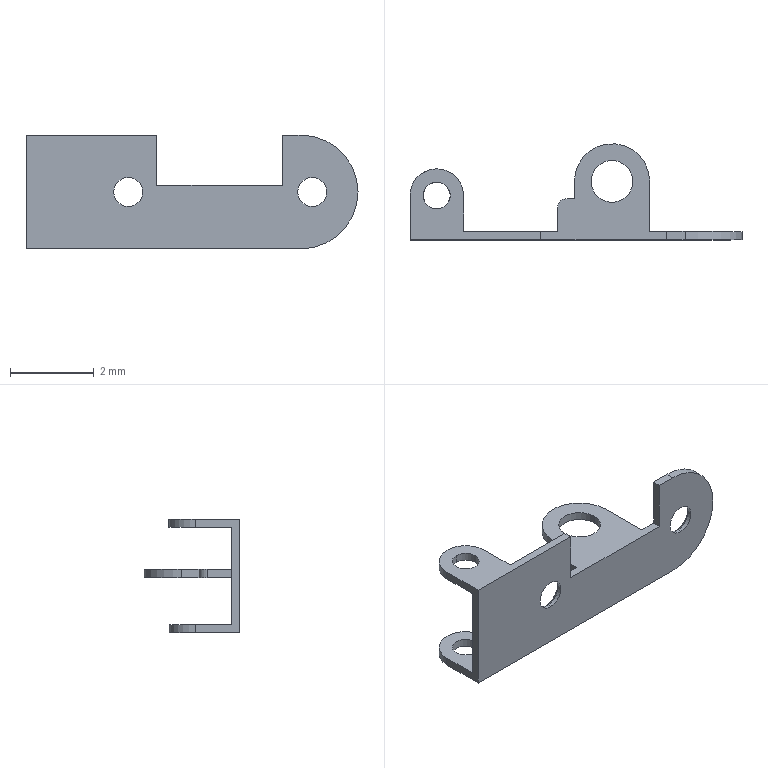Part | SolidWorks | features BaseBody 1, Scale 1 | 1 solid | 38 faces | box 7.94 x 2.3 x 2.72 mm | volume 4.422 mm3 | plane 18 | cylinder 16 | cone 4 | commonest cylinder face diameters 0.64 x4 0.7 x4 1.28 x3 1 x2 0.4 x1 1.8 x1
STEP:
#1=CARTESIAN_POINT('',(10.414,2.347,-1.823));
#2=VERTEX_POINT('',#1);
#3=CARTESIAN_POINT('',(9.774,2.347,-1.823));
#4=VERTEX_POINT('',#3);
#5=CARTESIAN_POINT('',(10.094,2.347,-1.823));
#6=DIRECTION('',(0.,0.,-1.));
#7=DIRECTION('',(1.,0.,0.));
#8=AXIS2_PLACEMENT_3D('',#5,#6,#7);
#9=CIRCLE('',#8,0.32);
#10=EDGE_CURVE('',#2,#4,#9,.T.);
#11=ORIENTED_EDGE('',*,*,#10,.T.);
#12=CARTESIAN_POINT('',(9.774,2.347,-1.623));
#13=VERTEX_POINT('',#12);
#14=CARTESIAN_POINT('',(9.774,2.347,-1.823));
#15=DIRECTION('',(0.,0.,1.));
#16=VECTOR('',#15,1000.);
#17=LINE('',#14,#16);
#18=EDGE_CURVE('',#4,#13,#17,.T.);
#19=ORIENTED_EDGE('',*,*,#18,.T.);
#20=CARTESIAN_POINT('',(10.414,2.347,-1.623));
#21=VERTEX_POINT('',#20);
#22=CARTESIAN_POINT('',(10.094,2.347,-1.623));
#23=DIRECTION('',(0.,0.,1.));
#24=DIRECTION('',(1.,0.,0.));
#25=AXIS2_PLACEMENT_3D('',#22,#23,#24);
#26=CIRCLE('',#25,0.32);
#27=EDGE_CURVE('',#13,#21,#26,.T.);
#28=ORIENTED_EDGE('',*,*,#27,.T.);
#29=CARTESIAN_POINT('',(10.414,2.347,-1.823));
#30=DIRECTION('',(0.,0.,1.));
#31=VECTOR('',#30,1000.);
#32=LINE('',#29,#31);
#33=EDGE_CURVE('',#2,#21,#32,.T.);
#34=ORIENTED_EDGE('',*,*,#33,.F.);
#35=EDGE_LOOP('',(#11,#19,#28,#34));
#36=FACE_OUTER_BOUND('',#35,.T.);
#37=CARTESIAN_POINT('',(10.094,2.347,-1.823));
#38=DIRECTION('',(0.,0.,1.));
#39=DIRECTION('',(1.,0.,0.));
#40=AXIS2_PLACEMENT_3D('',#37,#38,#39);
#41=CYLINDRICAL_SURFACE('',#40,0.32);
#42=ADVANCED_FACE('',(#36),#41,.F.);
#43=CARTESIAN_POINT('',(11.9,1.387,-0.113));
#44=VERTEX_POINT('',#43);
#45=CARTESIAN_POINT('',(11.9,1.387,-0.813));
#46=VERTEX_POINT('',#45);
#47=CARTESIAN_POINT('',(11.9,1.387,-0.463));
#48=DIRECTION('',(0.,-1.,0.));
#49=DIRECTION('',(0.,0.,1.));
#50=AXIS2_PLACEMENT_3D('',#47,#48,#49);
#51=CIRCLE('',#50,0.35);
#52=EDGE_CURVE('',#44,#46,#51,.T.);
#53=ORIENTED_EDGE('',*,*,#52,.T.);
#54=CARTESIAN_POINT('',(11.9,1.487,-0.913));
#55=VERTEX_POINT('',#54);
#56=CARTESIAN_POINT('',(11.9,1.387,-0.813));
#57=DIRECTION('',(0.,0.7071,-0.7071));
#58=VECTOR('',#57,1000.);
#59=LINE('',#56,#58);
#60=EDGE_CURVE('',#46,#55,#59,.T.);
#61=ORIENTED_EDGE('',*,*,#60,.T.);
#62=CARTESIAN_POINT('',(11.9,1.487,-0.013));
#63=VERTEX_POINT('',#62);
#64=CARTESIAN_POINT('',(11.9,1.487,-0.463));
#65=DIRECTION('',(0.,-1.,0.));
#66=DIRECTION('',(0.,0.,1.));
#67=AXIS2_PLACEMENT_3D('',#64,#65,#66);
#68=CIRCLE('',#67,0.45);
#69=EDGE_CURVE('',#63,#55,#68,.T.);
#70=ORIENTED_EDGE('',*,*,#69,.F.);
#71=CARTESIAN_POINT('',(11.9,1.387,-0.113));
#72=DIRECTION('',(0.,0.7071,0.7071));
#73=VECTOR('',#72,1000.);
#74=LINE('',#71,#73);
#75=EDGE_CURVE('',#44,#63,#74,.T.);
#76=ORIENTED_EDGE('',*,*,#75,.F.);
#77=EDGE_LOOP('',(#53,#61,#70,#76));
#78=FACE_OUTER_BOUND('',#77,.T.);
#79=CARTESIAN_POINT('',(11.9,1.387,-0.463));
#80=DIRECTION('',(0.,1.,0.));
#81=DIRECTION('',(0.,0.,1.));
#82=AXIS2_PLACEMENT_3D('',#79,#80,#81);
#83=CONICAL_SURFACE('',#82,0.35,0.7854);
#84=ADVANCED_FACE('',(#78),#83,.F.);
#85=CARTESIAN_POINT('',(16.3,1.387,-0.113));
#86=VERTEX_POINT('',#85);
#87=CARTESIAN_POINT('',(16.3,1.387,-0.813));
#88=VERTEX_POINT('',#87);
#89=CARTESIAN_POINT('',(16.3,1.387,-0.463));
#90=DIRECTION('',(0.,-1.,0.));
#91=DIRECTION('',(0.,0.,1.));
#92=AXIS2_PLACEMENT_3D('',#89,#90,#91);
#93=CIRCLE('',#92,0.35);
#94=EDGE_CURVE('',#86,#88,#93,.T.);
#95=ORIENTED_EDGE('',*,*,#94,.T.);
#96=CARTESIAN_POINT('',(16.3,1.487,-0.913));
#97=VERTEX_POINT('',#96);
#98=CARTESIAN_POINT('',(16.3,1.387,-0.813));
#99=DIRECTION('',(0.,0.7071,-0.7071));
#100=VECTOR('',#99,1000.);
#101=LINE('',#98,#100);
#102=EDGE_CURVE('',#88,#97,#101,.T.);
#103=ORIENTED_EDGE('',*,*,#102,.T.);
#104=CARTESIAN_POINT('',(16.3,1.487,-0.013));
#105=VERTEX_POINT('',#104);
#106=CARTESIAN_POINT('',(16.3,1.487,-0.463));
#107=DIRECTION('',(0.,-1.,0.));
#108=DIRECTION('',(0.,0.,1.));
#109=AXIS2_PLACEMENT_3D('',#106,#107,#108);
#110=CIRCLE('',#109,0.45);
#111=EDGE_CURVE('',#105,#97,#110,.T.);
#112=ORIENTED_EDGE('',*,*,#111,.F.);
#113=CARTESIAN_POINT('',(16.3,1.387,-0.113));
#114=DIRECTION('',(0.,0.7071,0.7071));
#115=VECTOR('',#114,1000.);
#116=LINE('',#113,#115);
#117=EDGE_CURVE('',#86,#105,#116,.T.);
#118=ORIENTED_EDGE('',*,*,#117,.F.);
#119=EDGE_LOOP('',(#95,#103,#112,#118));
#120=FACE_OUTER_BOUND('',#119,.T.);
#121=CARTESIAN_POINT('',(16.3,1.387,-0.463));
#122=DIRECTION('',(0.,1.,0.));
#123=DIRECTION('',(0.,0.,1.));
#124=AXIS2_PLACEMENT_3D('',#121,#122,#123);
#125=CONICAL_SURFACE('',#124,0.35,0.7854);
#126=ADVANCED_FACE('',(#120),#125,.F.);
#127=ORIENTED_EDGE('',*,*,#94,.F.);
#128=CARTESIAN_POINT('',(16.3,1.287,-0.113));
#129=VERTEX_POINT('',#128);
#130=CARTESIAN_POINT('',(16.3,1.387,-0.113));
#131=DIRECTION('',(0.,-1.,0.));
#132=VECTOR('',#131,1000.);
#133=LINE('',#130,#132);
#134=EDGE_CURVE('',#86,#129,#133,.T.);
#135=ORIENTED_EDGE('',*,*,#134,.T.);
#136=CARTESIAN_POINT('',(16.3,1.287,-0.813));
#137=VERTEX_POINT('',#136);
#138=CARTESIAN_POINT('',(16.3,1.287,-0.463));
#139=DIRECTION('',(0.,-1.,0.));
#140=DIRECTION('',(0.,0.,-1.));
#141=AXIS2_PLACEMENT_3D('',#138,#139,#140);
#142=CIRCLE('',#141,0.35);
#143=EDGE_CURVE('',#129,#137,#142,.T.);
#144=ORIENTED_EDGE('',*,*,#143,.T.);
#145=CARTESIAN_POINT('',(16.3,1.387,-0.813));
#146=DIRECTION('',(0.,-1.,0.));
#147=VECTOR('',#146,1000.);
#148=LINE('',#145,#147);
#149=EDGE_CURVE('',#88,#137,#148,.T.);
#150=ORIENTED_EDGE('',*,*,#149,.F.);
#151=EDGE_LOOP('',(#127,#135,#144,#150));
#152=FACE_OUTER_BOUND('',#151,.T.);
#153=CARTESIAN_POINT('',(16.3,1.387,-0.463));
#154=DIRECTION('',(0.,-1.,0.));
#155=DIRECTION('',(0.,0.,-1.));
#156=AXIS2_PLACEMENT_3D('',#153,#154,#155);
#157=CYLINDRICAL_SURFACE('',#156,0.35);
#158=ADVANCED_FACE('',(#152),#157,.F.);
#159=ORIENTED_EDGE('',*,*,#52,.F.);
#160=CARTESIAN_POINT('',(11.9,1.287,-0.113));
#161=VERTEX_POINT('',#160);
#162=CARTESIAN_POINT('',(11.9,1.387,-0.113));
#163=DIRECTION('',(0.,-1.,0.));
#164=VECTOR('',#163,1000.);
#165=LINE('',#162,#164);
#166=EDGE_CURVE('',#44,#161,#165,.T.);
#167=ORIENTED_EDGE('',*,*,#166,.T.);
#168=CARTESIAN_POINT('',(11.9,1.287,-0.813));
#169=VERTEX_POINT('',#168);
#170=CARTESIAN_POINT('',(11.9,1.287,-0.463));
#171=DIRECTION('',(0.,-1.,0.));
#172=DIRECTION('',(0.,0.,-1.));
#173=AXIS2_PLACEMENT_3D('',#170,#171,#172);
#174=CIRCLE('',#173,0.35);
#175=EDGE_CURVE('',#161,#169,#174,.T.);
#176=ORIENTED_EDGE('',*,*,#175,.T.);
#177=CARTESIAN_POINT('',(11.9,1.387,-0.813));
#178=DIRECTION('',(0.,-1.,0.));
#179=VECTOR('',#178,1000.);
#180=LINE('',#177,#179);
#181=EDGE_CURVE('',#46,#169,#180,.T.);
#182=ORIENTED_EDGE('',*,*,#181,.F.);
#183=EDGE_LOOP('',(#159,#167,#176,#182));
#184=FACE_OUTER_BOUND('',#183,.T.);
#185=CARTESIAN_POINT('',(11.9,1.387,-0.463));
#186=DIRECTION('',(0.,-1.,0.));
#187=DIRECTION('',(0.,0.,-1.));
#188=AXIS2_PLACEMENT_3D('',#185,#186,#187);
#189=CYLINDRICAL_SURFACE('',#188,0.35);
#190=ADVANCED_FACE('',(#184),#189,.F.);
#191=CARTESIAN_POINT('',(13.785,2.687,-0.503));
#192=VERTEX_POINT('',#191);
#193=CARTESIAN_POINT('',(14.785,2.687,-0.503));
#194=VERTEX_POINT('',#193);
#195=CARTESIAN_POINT('',(14.285,2.687,-0.503));
#196=DIRECTION('',(0.,0.,1.));
#197=DIRECTION('',(1.,0.,0.));
#198=AXIS2_PLACEMENT_3D('',#195,#196,#197);
#199=CIRCLE('',#198,0.5);
#200=EDGE_CURVE('',#192,#194,#199,.T.);
#201=ORIENTED_EDGE('',*,*,#200,.F.);
#202=CARTESIAN_POINT('',(13.785,2.687,-0.303));
#203=VERTEX_POINT('',#202);
#204=CARTESIAN_POINT('',(13.785,2.687,-0.503));
#205=DIRECTION('',(0.,0.,1.));
#206=VECTOR('',#205,1000.);
#207=LINE('',#204,#206);
#208=EDGE_CURVE('',#192,#203,#207,.T.);
#209=ORIENTED_EDGE('',*,*,#208,.T.);
#210=CARTESIAN_POINT('',(14.785,2.687,-0.303));
#211=VERTEX_POINT('',#210);
#212=CARTESIAN_POINT('',(14.285,2.687,-0.303));
#213=DIRECTION('',(0.,0.,1.));
#214=DIRECTION('',(1.,0.,0.));
#215=AXIS2_PLACEMENT_3D('',#212,#213,#214);
#216=CIRCLE('',#215,0.5);
#217=EDGE_CURVE('',#203,#211,#216,.T.);
#218=ORIENTED_EDGE('',*,*,#217,.T.);
#219=CARTESIAN_POINT('',(14.785,2.687,-0.503));
#220=DIRECTION('',(0.,0.,1.));
#221=VECTOR('',#220,1000.);
#222=LINE('',#219,#221);
#223=EDGE_CURVE('',#194,#211,#222,.T.);
#224=ORIENTED_EDGE('',*,*,#223,.F.);
#225=EDGE_LOOP('',(#201,#209,#218,#224));
#226=FACE_OUTER_BOUND('',#225,.T.);
#227=CARTESIAN_POINT('',(14.285,2.687,-0.503));
#228=DIRECTION('',(0.,0.,1.));
#229=DIRECTION('',(1.,0.,0.));
#230=AXIS2_PLACEMENT_3D('',#227,#228,#229);
#231=CYLINDRICAL_SURFACE('',#230,0.5);
#232=ADVANCED_FACE('',(#226),#231,.F.);
#233=CARTESIAN_POINT('',(10.094,2.667,0.897));
#234=VERTEX_POINT('',#233);
#235=CARTESIAN_POINT('',(10.094,2.027,0.897));
#236=VERTEX_POINT('',#235);
#237=CARTESIAN_POINT('',(10.094,2.347,0.897));
#238=DIRECTION('',(0.,0.,1.));
#239=DIRECTION('',(0.,1.,0.));
#240=AXIS2_PLACEMENT_3D('',#237,#238,#239);
#241=CIRCLE('',#240,0.32);
#242=EDGE_CURVE('',#234,#236,#241,.T.);
#243=ORIENTED_EDGE('',*,*,#242,.T.);
#244=CARTESIAN_POINT('',(10.094,2.027,0.697));
#245=VERTEX_POINT('',#244);
#246=CARTESIAN_POINT('',(10.094,2.027,0.897));
#247=DIRECTION('',(0.,0.,-1.));
#248=VECTOR('',#247,1000.);
#249=LINE('',#246,#248);
#250=EDGE_CURVE('',#236,#245,#249,.T.);
#251=ORIENTED_EDGE('',*,*,#250,.T.);
#252=CARTESIAN_POINT('',(10.094,2.667,0.697));
#253=VERTEX_POINT('',#252);
#254=CARTESIAN_POINT('',(10.094,2.347,0.697));
#255=DIRECTION('',(0.,0.,1.));
#256=DIRECTION('',(0.,1.,0.));
#257=AXIS2_PLACEMENT_3D('',#254,#255,#256);
#258=CIRCLE('',#257,0.32);
#259=EDGE_CURVE('',#253,#245,#258,.T.);
#260=ORIENTED_EDGE('',*,*,#259,.F.);
#261=CARTESIAN_POINT('',(10.094,2.667,0.897));
#262=DIRECTION('',(0.,0.,-1.));
#263=VECTOR('',#262,1000.);
#264=LINE('',#261,#263);
#265=EDGE_CURVE('',#234,#253,#264,.T.);
#266=ORIENTED_EDGE('',*,*,#265,.F.);
#267=EDGE_LOOP('',(#243,#251,#260,#266));
#268=FACE_OUTER_BOUND('',#267,.T.);
#269=CARTESIAN_POINT('',(10.094,2.347,0.897));
#270=DIRECTION('',(0.,0.,-1.));
#271=DIRECTION('',(0.,1.,0.));
#272=AXIS2_PLACEMENT_3D('',#269,#270,#271);
#273=CYLINDRICAL_SURFACE('',#272,0.32);
#274=ADVANCED_FACE('',(#268),#273,.F.);
#275=CARTESIAN_POINT('',(9.454,2.347,0.897));
#276=VERTEX_POINT('',#275);
#277=CARTESIAN_POINT('',(10.094,2.987,0.897));
#278=VERTEX_POINT('',#277);
#279=CARTESIAN_POINT('',(10.094,2.347,0.897));
#280=DIRECTION('',(0.,0.,-1.));
#281=DIRECTION('',(0.,1.,0.));
#282=AXIS2_PLACEMENT_3D('',#279,#280,#281);
#283=CIRCLE('',#282,0.64);
#284=EDGE_CURVE('',#276,#278,#283,.T.);
#285=ORIENTED_EDGE('',*,*,#284,.T.);
#286=CARTESIAN_POINT('',(10.094,2.987,0.697));
#287=VERTEX_POINT('',#286);
#288=CARTESIAN_POINT('',(10.094,2.987,0.897));
#289=DIRECTION('',(0.,0.,-1.));
#290=VECTOR('',#289,1000.);
#291=LINE('',#288,#290);
#292=EDGE_CURVE('',#278,#287,#291,.T.);
#293=ORIENTED_EDGE('',*,*,#292,.T.);
#294=CARTESIAN_POINT('',(9.454,2.347,0.697));
#295=VERTEX_POINT('',#294);
#296=CARTESIAN_POINT('',(10.094,2.347,0.697));
#297=DIRECTION('',(0.,0.,-1.));
#298=DIRECTION('',(0.,1.,0.));
#299=AXIS2_PLACEMENT_3D('',#296,#297,#298);
#300=CIRCLE('',#299,0.64);
#301=EDGE_CURVE('',#295,#287,#300,.T.);
#302=ORIENTED_EDGE('',*,*,#301,.F.);
#303=CARTESIAN_POINT('',(9.454,2.347,0.797));
#304=DIRECTION('',(0.,0.,-1.));
#305=VECTOR('',#304,1000.);
#306=LINE('',#303,#305);
#307=EDGE_CURVE('',#276,#295,#306,.T.);
#308=ORIENTED_EDGE('',*,*,#307,.F.);
#309=EDGE_LOOP('',(#285,#293,#302,#308));
#310=FACE_OUTER_BOUND('',#309,.T.);
#311=CARTESIAN_POINT('',(10.094,2.347,0.897));
#312=DIRECTION('',(0.,0.,-1.));
#313=DIRECTION('',(0.,1.,0.));
#314=AXIS2_PLACEMENT_3D('',#311,#312,#313);
#315=CYLINDRICAL_SURFACE('',#314,0.64);
#316=ADVANCED_FACE('',(#310),#315,.T.);
#317=ORIENTED_EDGE('',*,*,#18,.F.);
#318=CARTESIAN_POINT('',(10.094,2.347,-1.823));
#319=DIRECTION('',(0.,0.,-1.));
#320=DIRECTION('',(1.,0.,0.));
#321=AXIS2_PLACEMENT_3D('',#318,#319,#320);
#322=CIRCLE('',#321,0.32);
#323=EDGE_CURVE('',#4,#2,#322,.T.);
#324=ORIENTED_EDGE('',*,*,#323,.T.);
#325=ORIENTED_EDGE('',*,*,#33,.T.);
#326=CARTESIAN_POINT('',(10.094,2.347,-1.623));
#327=DIRECTION('',(0.,0.,1.));
#328=DIRECTION('',(1.,0.,0.));
#329=AXIS2_PLACEMENT_3D('',#326,#327,#328);
#330=CIRCLE('',#329,0.32);
#331=EDGE_CURVE('',#21,#13,#330,.T.);
#332=ORIENTED_EDGE('',*,*,#331,.T.);
#333=EDGE_LOOP('',(#317,#324,#325,#332));
#334=FACE_OUTER_BOUND('',#333,.T.);
#335=CARTESIAN_POINT('',(10.094,2.347,-1.823));
#336=DIRECTION('',(0.,0.,1.));
#337=DIRECTION('',(1.,0.,0.));
#338=AXIS2_PLACEMENT_3D('',#335,#336,#337);
#339=CYLINDRICAL_SURFACE('',#338,0.32);
#340=ADVANCED_FACE('',(#334),#339,.F.);
#341=ORIENTED_EDGE('',*,*,#331,.F.);
#342=ORIENTED_EDGE('',*,*,#27,.F.);
#343=EDGE_LOOP('',(#341,#342));
#344=FACE_BOUND('',#343,.T.);
#345=CARTESIAN_POINT('',(9.454,2.347,-1.623));
#346=VERTEX_POINT('',#345);
#347=CARTESIAN_POINT('',(9.454,1.487,-1.623));
#348=VERTEX_POINT('',#347);
#349=CARTESIAN_POINT('',(9.454,2.241,-1.623));
#350=DIRECTION('',(0.,-1.,0.));
#351=VECTOR('',#350,1000.);
#352=LINE('',#349,#351);
#353=EDGE_CURVE('',#346,#348,#352,.T.);
#354=ORIENTED_EDGE('',*,*,#353,.T.);
#355=CARTESIAN_POINT('',(10.734,1.487,-1.623));
#356=VERTEX_POINT('',#355);
#357=CARTESIAN_POINT('',(10.094,1.487,-1.623));
#358=DIRECTION('',(1.,0.,0.));
#359=VECTOR('',#358,1000.);
#360=LINE('',#357,#359);
#361=EDGE_CURVE('',#348,#356,#360,.T.);
#362=ORIENTED_EDGE('',*,*,#361,.T.);
#363=CARTESIAN_POINT('',(10.734,2.347,-1.623));
#364=VERTEX_POINT('',#363);
#365=CARTESIAN_POINT('',(10.734,2.241,-1.623));
#366=DIRECTION('',(0.,1.,0.));
#367=VECTOR('',#366,1000.);
#368=LINE('',#365,#367);
#369=EDGE_CURVE('',#356,#364,#368,.T.);
#370=ORIENTED_EDGE('',*,*,#369,.T.);
#371=CARTESIAN_POINT('',(10.094,2.347,-1.623));
#372=DIRECTION('',(0.,0.,1.));
#373=DIRECTION('',(1.,0.,0.));
#374=AXIS2_PLACEMENT_3D('',#371,#372,#373);
#375=CIRCLE('',#374,0.64);
#376=EDGE_CURVE('',#364,#346,#375,.T.);
#377=ORIENTED_EDGE('',*,*,#376,.T.);
#378=EDGE_LOOP('',(#354,#362,#370,#377));
#379=FACE_OUTER_BOUND('',#378,.T.);
#380=CARTESIAN_POINT('',(9.454,2.996,-1.623));
#381=DIRECTION('',(0.,0.,1.));
#382=DIRECTION('',(0.,-1.,0.));
#383=AXIS2_PLACEMENT_3D('',#380,#381,#382);
#384=PLANE('',#383);
#385=ADVANCED_FACE('',(#344,#379),#384,.T.);
#386=ORIENTED_EDGE('',*,*,#10,.F.);
#387=ORIENTED_EDGE('',*,*,#323,.F.);
#388=EDGE_LOOP('',(#386,#387));
#389=FACE_BOUND('',#388,.T.);
#390=CARTESIAN_POINT('',(9.454,2.347,-1.823));
#391=VERTEX_POINT('',#390);
#392=CARTESIAN_POINT('',(9.454,1.287,-1.823));
#393=VERTEX_POINT('',#392);
#394=CARTESIAN_POINT('',(9.454,2.142,-1.823));
#395=DIRECTION('',(0.,-1.,0.));
#396=VECTOR('',#395,1000.);
#397=LINE('',#394,#396);
#398=EDGE_CURVE('',#391,#393,#397,.T.);
#399=ORIENTED_EDGE('',*,*,#398,.F.);
#400=CARTESIAN_POINT('',(10.734,2.347,-1.823));
#401=VERTEX_POINT('',#400);
#402=CARTESIAN_POINT('',(10.094,2.347,-1.823));
#403=DIRECTION('',(0.,0.,1.));
#404=DIRECTION('',(1.,0.,0.));
#405=AXIS2_PLACEMENT_3D('',#402,#403,#404);
#406=CIRCLE('',#405,0.64);
#407=EDGE_CURVE('',#401,#391,#406,.T.);
#408=ORIENTED_EDGE('',*,*,#407,.F.);
#409=CARTESIAN_POINT('',(10.734,1.487,-1.823));
#410=VERTEX_POINT('',#409);
#411=CARTESIAN_POINT('',(10.734,2.142,-1.823));
#412=DIRECTION('',(0.,1.,0.));
#413=VECTOR('',#412,1000.);
#414=LINE('',#411,#413);
#415=EDGE_CURVE('',#410,#401,#414,.T.);
#416=ORIENTED_EDGE('',*,*,#415,.F.);
#417=CARTESIAN_POINT('',(16.034,1.487,-1.823));
#418=VERTEX_POINT('',#417);
#419=CARTESIAN_POINT('',(12.744,1.487,-1.823));
#420=DIRECTION('',(-1.,0.,0.));
#421=VECTOR('',#420,1000.);
#422=LINE('',#419,#421);
#423=EDGE_CURVE('',#418,#410,#422,.T.);
#424=ORIENTED_EDGE('',*,*,#423,.F.);
#425=CARTESIAN_POINT('',(16.034,1.287,-1.823));
#426=VERTEX_POINT('',#425);
#427=CARTESIAN_POINT('',(16.034,1.387,-1.823));
#428=DIRECTION('',(0.,-1.,0.));
#429=VECTOR('',#428,1000.);
#430=LINE('',#427,#429);
#431=EDGE_CURVE('',#418,#426,#430,.T.);
#432=ORIENTED_EDGE('',*,*,#431,.T.);
#433=CARTESIAN_POINT('',(12.744,1.287,-1.823));
#434=DIRECTION('',(1.,0.,0.));
#435=VECTOR('',#434,1000.);
#436=LINE('',#433,#435);
#437=EDGE_CURVE('',#393,#426,#436,.T.);
#438=ORIENTED_EDGE('',*,*,#437,.F.);
#439=EDGE_LOOP('',(#399,#408,#416,#424,#432,#438));
#440=FACE_OUTER_BOUND('',#439,.T.);
#441=CARTESIAN_POINT('',(9.454,1.287,-1.823));
#442=DIRECTION('',(0.,0.,1.));
#443=DIRECTION('',(1.,0.,0.));
#444=AXIS2_PLACEMENT_3D('',#441,#442,#443);
#445=PLANE('',#444);
#446=ADVANCED_FACE('',(#389,#440),#445,.F.);
#447=ORIENTED_EDGE('',*,*,#69,.T.);
#448=CARTESIAN_POINT('',(11.9,1.487,-0.463));
#449=DIRECTION('',(0.,-1.,0.));
#450=DIRECTION('',(0.,0.,1.));
#451=AXIS2_PLACEMENT_3D('',#448,#449,#450);
#452=CIRCLE('',#451,0.45);
#453=EDGE_CURVE('',#55,#63,#452,.T.);
#454=ORIENTED_EDGE('',*,*,#453,.T.);
#455=EDGE_LOOP('',(#447,#454));
#456=FACE_BOUND('',#455,.T.);
#457=ORIENTED_EDGE('',*,*,#111,.T.);
#458=CARTESIAN_POINT('',(16.3,1.487,-0.463));
#459=DIRECTION('',(0.,-1.,0.));
#460=DIRECTION('',(0.,0.,1.));
#461=AXIS2_PLACEMENT_3D('',#458,#459,#460);
#462=CIRCLE('',#461,0.45);
#463=EDGE_CURVE('',#97,#105,#462,.T.);
#464=ORIENTED_EDGE('',*,*,#463,.T.);
#465=EDGE_LOOP('',(#457,#464));
#466=FACE_BOUND('',#465,.T.);
#467=CARTESIAN_POINT('',(12.584,1.487,-0.303));
#468=VERTEX_POINT('',#467);
#469=CARTESIAN_POINT('',(12.984,1.487,-0.303));
#470=VERTEX_POINT('',#469);
#471=CARTESIAN_POINT('',(13.448,1.487,-0.303));
#472=DIRECTION('',(1.,0.,0.));
#473=VECTOR('',#472,1000.);
#474=LINE('',#471,#473);
#475=EDGE_CURVE('',#468,#470,#474,.T.);
#476=ORIENTED_EDGE('',*,*,#475,.T.);
#477=CARTESIAN_POINT('',(12.984,1.487,-0.503));
#478=VERTEX_POINT('',#477);
#479=CARTESIAN_POINT('',(12.984,1.487,-0.403));
#480=DIRECTION('',(0.,0.,-1.));
#481=VECTOR('',#480,1000.);
#482=LINE('',#479,#481);
#483=EDGE_CURVE('',#470,#478,#482,.T.);
#484=ORIENTED_EDGE('',*,*,#483,.T.);
#485=CARTESIAN_POINT('',(15.184,1.487,-0.503));
#486=VERTEX_POINT('',#485);
#487=CARTESIAN_POINT('',(13.448,1.487,-0.503));
#488=DIRECTION('',(1.,0.,0.));
#489=VECTOR('',#488,1000.);
#490=LINE('',#487,#489);
#491=EDGE_CURVE('',#478,#486,#490,.T.);
#492=ORIENTED_EDGE('',*,*,#491,.T.);
#493=CARTESIAN_POINT('',(15.184,1.487,-0.303));
#494=VERTEX_POINT('',#493);
#495=CARTESIAN_POINT('',(15.184,1.487,-0.403));
#496=DIRECTION('',(0.,0.,-1.));
#497=VECTOR('',#496,1000.);
#498=LINE('',#495,#497);
#499=EDGE_CURVE('',#494,#486,#498,.T.);
#500=ORIENTED_EDGE('',*,*,#499,.F.);
#501=CARTESIAN_POINT('',(15.584,1.487,-0.303));
#502=VERTEX_POINT('',#501);
#503=CARTESIAN_POINT('',(13.448,1.487,-0.303));
#504=DIRECTION('',(1.,0.,0.));
#505=VECTOR('',#504,1000.);
#506=LINE('',#503,#505);
#507=EDGE_CURVE('',#494,#502,#506,.T.);
#508=ORIENTED_EDGE('',*,*,#507,.T.);
#509=CARTESIAN_POINT('',(15.584,1.487,0.897));
#510=VERTEX_POINT('',#509);
#511=CARTESIAN_POINT('',(15.584,1.487,-0.463));
#512=DIRECTION('',(0.,0.,1.));
#513=VECTOR('',#512,1000.);
#514=LINE('',#511,#513);
#515=EDGE_CURVE('',#502,#510,#514,.T.);
#516=ORIENTED_EDGE('',*,*,#515,.T.);
#517=CARTESIAN_POINT('',(16.034,1.487,0.897));
#518=VERTEX_POINT('',#517);
#519=CARTESIAN_POINT('',(13.448,1.487,0.897));
#520=DIRECTION('',(1.,0.,0.));
#521=VECTOR('',#520,1000.);
#522=LINE('',#519,#521);
#523=EDGE_CURVE('',#510,#518,#522,.T.);
#524=ORIENTED_EDGE('',*,*,#523,.T.);
#525=CARTESIAN_POINT('',(16.034,1.487,-0.463));
#526=DIRECTION('',(0.,1.,0.));
#527=DIRECTION('',(0.,0.,-1.));
#528=AXIS2_PLACEMENT_3D('',#525,#526,#527);
#529=CIRCLE('',#528,1.36);
#530=EDGE_CURVE('',#518,#418,#529,.T.);
#531=ORIENTED_EDGE('',*,*,#530,.T.);
#532=ORIENTED_EDGE('',*,*,#423,.T.);
#533=CARTESIAN_POINT('',(10.734,1.487,-0.463));
#534=DIRECTION('',(0.,0.,1.));
#535=VECTOR('',#534,1000.);
#536=LINE('',#533,#535);
#537=EDGE_CURVE('',#410,#356,#536,.T.);
#538=ORIENTED_EDGE('',*,*,#537,.T.);
#539=ORIENTED_EDGE('',*,*,#361,.F.);
#540=CARTESIAN_POINT('',(9.454,1.487,0.697));
#541=VERTEX_POINT('',#540);
#542=CARTESIAN_POINT('',(9.454,1.487,-0.463));
#543=DIRECTION('',(0.,0.,1.));
#544=VECTOR('',#543,1000.);
#545=LINE('',#542,#544);
#546=EDGE_CURVE('',#348,#541,#545,.T.);
#547=ORIENTED_EDGE('',*,*,#546,.T.);
#548=CARTESIAN_POINT('',(10.734,1.487,0.697));
#549=VERTEX_POINT('',#548);
#550=CARTESIAN_POINT('',(13.448,1.487,0.697));
#551=DIRECTION('',(1.,0.,0.));
#552=VECTOR('',#551,1000.);
#553=LINE('',#550,#552);
#554=EDGE_CURVE('',#541,#549,#553,.T.);
#555=ORIENTED_EDGE('',*,*,#554,.T.);
#556=CARTESIAN_POINT('',(10.734,1.487,0.897));
#557=VERTEX_POINT('',#556);
#558=CARTESIAN_POINT('',(10.734,1.487,0.797));
#559=DIRECTION('',(0.,0.,1.));
#560=VECTOR('',#559,1000.);
#561=LINE('',#558,#560);
#562=EDGE_CURVE('',#549,#557,#561,.T.);
#563=ORIENTED_EDGE('',*,*,#562,.T.);
#564=CARTESIAN_POINT('',(12.584,1.487,0.897));
#565=VERTEX_POINT('',#564);
#566=CARTESIAN_POINT('',(13.448,1.487,0.897));
#567=DIRECTION('',(1.,0.,0.));
#568=VECTOR('',#567,1000.);
#569=LINE('',#566,#568);
#570=EDGE_CURVE('',#557,#565,#569,.T.);
#571=ORIENTED_EDGE('',*,*,#570,.T.);
#572=CARTESIAN_POINT('',(12.584,1.487,-0.463));
#573=DIRECTION('',(0.,0.,-1.));
#574=VECTOR('',#573,1000.);
#575=LINE('',#572,#574);
#576=EDGE_CURVE('',#565,#468,#575,.T.);
#577=ORIENTED_EDGE('',*,*,#576,.T.);
#578=EDGE_LOOP('',(#476,#484,#492,#500,#508,#516,#524,#531,#532,#538,#539,#547,#555,#563,#571,#577));
#579=FACE_OUTER_BOUND('',#578,.T.);
#580=CARTESIAN_POINT('',(9.454,1.487,-1.823));
#581=DIRECTION('',(0.,1.,0.));
#582=DIRECTION('',(0.,0.,1.));
#583=AXIS2_PLACEMENT_3D('',#580,#581,#582);
#584=PLANE('',#583);
#585=ADVANCED_FACE('',(#456,#466,#579),#584,.T.);
#586=ORIENTED_EDGE('',*,*,#546,.F.);
#587=ORIENTED_EDGE('',*,*,#353,.F.);
#588=CARTESIAN_POINT('',(9.454,2.347,-0.463));
#589=DIRECTION('',(0.,0.,1.));
#590=VECTOR('',#589,1000.);
#591=LINE('',#588,#590);
#592=EDGE_CURVE('',#391,#346,#591,.T.);
#593=ORIENTED_EDGE('',*,*,#592,.F.);
#594=ORIENTED_EDGE('',*,*,#398,.T.);
#595=CARTESIAN_POINT('',(9.454,1.287,0.897));
#596=VERTEX_POINT('',#595);
#597=CARTESIAN_POINT('',(9.454,1.287,-0.463));
#598=DIRECTION('',(0.,0.,-1.));
#599=VECTOR('',#598,1000.);
#600=LINE('',#597,#599);
#601=EDGE_CURVE('',#596,#393,#600,.T.);
#602=ORIENTED_EDGE('',*,*,#601,.F.);
#603=CARTESIAN_POINT('',(9.454,1.817,0.897));
#604=DIRECTION('',(0.,-1.,0.));
#605=VECTOR('',#604,1000.);
#606=LINE('',#603,#605);
#607=EDGE_CURVE('',#276,#596,#606,.T.);
#608=ORIENTED_EDGE('',*,*,#607,.F.);
#609=ORIENTED_EDGE('',*,*,#307,.T.);
#610=CARTESIAN_POINT('',(9.454,1.817,0.697));
#611=DIRECTION('',(0.,1.,0.));
#612=VECTOR('',#611,1000.);
#613=LINE('',#610,#612);
#614=EDGE_CURVE('',#541,#295,#613,.T.);
#615=ORIENTED_EDGE('',*,*,#614,.F.);
#616=EDGE_LOOP('',(#586,#587,#593,#594,#602,#608,#609,#615));
#617=FACE_OUTER_BOUND('',#616,.T.);
#618=CARTESIAN_POINT('',(9.454,1.287,0.897));
#619=DIRECTION('',(1.,0.,0.));
#620=DIRECTION('',(0.,0.,-1.));
#621=AXIS2_PLACEMENT_3D('',#618,#619,#620);
#622=PLANE('',#621);
#623=ADVANCED_FACE('',(#617),#622,.F.);
#624=CARTESIAN_POINT('',(10.734,2.347,-1.723));
#625=DIRECTION('',(0.,0.,1.));
#626=VECTOR('',#625,1000.);
#627=LINE('',#624,#626);
#628=EDGE_CURVE('',#401,#364,#627,.T.);
#629=ORIENTED_EDGE('',*,*,#628,.F.);
#630=ORIENTED_EDGE('',*,*,#407,.T.);
#631=ORIENTED_EDGE('',*,*,#592,.T.);
#632=ORIENTED_EDGE('',*,*,#376,.F.);
#633=EDGE_LOOP('',(#629,#630,#631,#632));
#634=FACE_OUTER_BOUND('',#633,.T.);
#635=CARTESIAN_POINT('',(10.094,2.347,-1.823));
#636=DIRECTION('',(0.,0.,1.));
#637=DIRECTION('',(1.,0.,0.));
#638=AXIS2_PLACEMENT_3D('',#635,#636,#637);
#639=CYLINDRICAL_SURFACE('',#638,0.64);
#640=ADVANCED_FACE('',(#634),#639,.T.);
#641=ORIENTED_EDGE('',*,*,#537,.F.);
#642=ORIENTED_EDGE('',*,*,#415,.T.);
#643=ORIENTED_EDGE('',*,*,#628,.T.);
#644=ORIENTED_EDGE('',*,*,#369,.F.);
#645=EDGE_LOOP('',(#641,#642,#643,#644));
#646=FACE_OUTER_BOUND('',#645,.T.);
#647=CARTESIAN_POINT('',(10.734,2.347,-1.823));
#648=DIRECTION('',(-1.,0.,0.));
#649=DIRECTION('',(0.,-1.,0.));
#650=AXIS2_PLACEMENT_3D('',#647,#648,#649);
#651=PLANE('',#650);
#652=ADVANCED_FACE('',(#646),#651,.F.);
#653=CARTESIAN_POINT('',(16.3,1.287,-0.463));
#654=DIRECTION('',(0.,-1.,0.));
#655=DIRECTION('',(0.,0.,-1.));
#656=AXIS2_PLACEMENT_3D('',#653,#654,#655);
#657=CIRCLE('',#656,0.35);
#658=EDGE_CURVE('',#137,#129,#657,.T.);
#659=ORIENTED_EDGE('',*,*,#658,.F.);
#660=ORIENTED_EDGE('',*,*,#143,.F.);
#661=EDGE_LOOP('',(#659,#660));
#662=FACE_BOUND('',#661,.T.);
#663=CARTESIAN_POINT('',(11.9,1.287,-0.463));
#664=DIRECTION('',(0.,-1.,0.));
#665=DIRECTION('',(0.,0.,-1.));
#666=AXIS2_PLACEMENT_3D('',#663,#664,#665);
#667=CIRCLE('',#666,0.35);
#668=EDGE_CURVE('',#169,#161,#667,.T.);
#669=ORIENTED_EDGE('',*,*,#668,.F.);
#670=ORIENTED_EDGE('',*,*,#175,.F.);
#671=EDGE_LOOP('',(#669,#670));
#672=FACE_BOUND('',#671,.T.);
#673=CARTESIAN_POINT('',(12.584,1.287,0.897));
#674=VERTEX_POINT('',#673);
#675=CARTESIAN_POINT('',(12.584,1.287,-0.303));
#676=VERTEX_POINT('',#675);
#677=CARTESIAN_POINT('',(12.584,1.287,-0.463));
#678=DIRECTION('',(0.,0.,-1.));
#679=VECTOR('',#678,1000.);
#680=LINE('',#677,#679);
#681=EDGE_CURVE('',#674,#676,#680,.T.);
#682=ORIENTED_EDGE('',*,*,#681,.F.);
#683=CARTESIAN_POINT('',(13.448,1.287,0.897));
#684=DIRECTION('',(1.,0.,0.));
#685=VECTOR('',#684,1000.);
#686=LINE('',#683,#685);
#687=EDGE_CURVE('',#596,#674,#686,.T.);
#688=ORIENTED_EDGE('',*,*,#687,.F.);
#689=ORIENTED_EDGE('',*,*,#601,.T.);
#690=ORIENTED_EDGE('',*,*,#437,.T.);
#691=CARTESIAN_POINT('',(16.034,1.287,0.897));
#692=VERTEX_POINT('',#691);
#693=CARTESIAN_POINT('',(16.034,1.287,-0.463));
#694=DIRECTION('',(0.,1.,0.));
#695=DIRECTION('',(0.,0.,-1.));
#696=AXIS2_PLACEMENT_3D('',#693,#694,#695);
#697=CIRCLE('',#696,1.36);
#698=EDGE_CURVE('',#692,#426,#697,.T.);
#699=ORIENTED_EDGE('',*,*,#698,.F.);
#700=CARTESIAN_POINT('',(15.584,1.287,0.897));
#701=VERTEX_POINT('',#700);
#702=CARTESIAN_POINT('',(13.448,1.287,0.897));
#703=DIRECTION('',(1.,0.,0.));
#704=VECTOR('',#703,1000.);
#705=LINE('',#702,#704);
#706=EDGE_CURVE('',#701,#692,#705,.T.);
#707=ORIENTED_EDGE('',*,*,#706,.F.);
#708=CARTESIAN_POINT('',(15.584,1.287,-0.303));
#709=VERTEX_POINT('',#708);
#710=CARTESIAN_POINT('',(15.584,1.287,-0.463));
#711=DIRECTION('',(0.,0.,1.));
#712=VECTOR('',#711,1000.);
#713=LINE('',#710,#712);
#714=EDGE_CURVE('',#709,#701,#713,.T.);
#715=ORIENTED_EDGE('',*,*,#714,.F.);
#716=CARTESIAN_POINT('',(13.448,1.287,-0.303));
#717=DIRECTION('',(1.,0.,0.));
#718=VECTOR('',#717,1000.);
#719=LINE('',#716,#718);
#720=EDGE_CURVE('',#676,#709,#719,.T.);
#721=ORIENTED_EDGE('',*,*,#720,.F.);
#722=EDGE_LOOP('',(#682,#688,#689,#690,#699,#707,#715,#721));
#723=FACE_OUTER_BOUND('',#722,.T.);
#724=CARTESIAN_POINT('',(9.454,1.287,-1.823));
#725=DIRECTION('',(0.,1.,0.));
#726=DIRECTION('',(0.,0.,1.));
#727=AXIS2_PLACEMENT_3D('',#724,#725,#726);
#728=PLANE('',#727);
#729=ADVANCED_FACE('',(#662,#672,#723),#728,.F.);
#730=ORIENTED_EDGE('',*,*,#60,.F.);
#731=CARTESIAN_POINT('',(11.9,1.387,-0.463));
#732=DIRECTION('',(0.,-1.,0.));
#733=DIRECTION('',(0.,0.,1.));
#734=AXIS2_PLACEMENT_3D('',#731,#732,#733);
#735=CIRCLE('',#734,0.35);
#736=EDGE_CURVE('',#46,#44,#735,.T.);
#737=ORIENTED_EDGE('',*,*,#736,.T.);
#738=ORIENTED_EDGE('',*,*,#75,.T.);
#739=ORIENTED_EDGE('',*,*,#453,.F.);
#740=EDGE_LOOP('',(#730,#737,#738,#739));
#741=FACE_OUTER_BOUND('',#740,.T.);
#742=CARTESIAN_POINT('',(11.9,1.387,-0.463));
#743=DIRECTION('',(0.,1.,0.));
#744=DIRECTION('',(0.,0.,1.));
#745=AXIS2_PLACEMENT_3D('',#742,#743,#744);
#746=CONICAL_SURFACE('',#745,0.35,0.7854);
#747=ADVANCED_FACE('',(#741),#746,.F.);
#748=ORIENTED_EDGE('',*,*,#102,.F.);
#749=CARTESIAN_POINT('',(16.3,1.387,-0.463));
#750=DIRECTION('',(0.,-1.,0.));
#751=DIRECTION('',(0.,0.,1.));
#752=AXIS2_PLACEMENT_3D('',#749,#750,#751);
#753=CIRCLE('',#752,0.35);
#754=EDGE_CURVE('',#88,#86,#753,.T.);
#755=ORIENTED_EDGE('',*,*,#754,.T.);
#756=ORIENTED_EDGE('',*,*,#117,.T.);
#757=ORIENTED_EDGE('',*,*,#463,.F.);
#758=EDGE_LOOP('',(#748,#755,#756,#757));
#759=FACE_OUTER_BOUND('',#758,.T.);
#760=CARTESIAN_POINT('',(16.3,1.387,-0.463));
#761=DIRECTION('',(0.,1.,0.));
#762=DIRECTION('',(0.,0.,1.));
#763=AXIS2_PLACEMENT_3D('',#760,#761,#762);
#764=CONICAL_SURFACE('',#763,0.35,0.7854);
#765=ADVANCED_FACE('',(#759),#764,.F.);
#766=CARTESIAN_POINT('',(14.285,2.687,-0.303));
#767=DIRECTION('',(0.,0.,1.));
#768=DIRECTION('',(1.,0.,0.));
#769=AXIS2_PLACEMENT_3D('',#766,#767,#768);
#770=CIRCLE('',#769,0.5);
#771=EDGE_CURVE('',#211,#203,#770,.T.);
#772=ORIENTED_EDGE('',*,*,#771,.F.);
#773=ORIENTED_EDGE('',*,*,#217,.F.);
#774=EDGE_LOOP('',(#772,#773));
#775=FACE_BOUND('',#774,.T.);
#776=CARTESIAN_POINT('',(12.984,2.067,-0.303));
#777=VERTEX_POINT('',#776);
#778=CARTESIAN_POINT('',(13.184,2.267,-0.303));
#779=VERTEX_POINT('',#778);
#780=CARTESIAN_POINT('',(13.184,2.067,-0.303));
#781=DIRECTION('',(0.,0.,-1.));
#782=DIRECTION('',(-1.,0.,0.));
#783=AXIS2_PLACEMENT_3D('',#780,#781,#782);
#784=CIRCLE('',#783,0.2);
#785=EDGE_CURVE('',#777,#779,#784,.T.);
#786=ORIENTED_EDGE('',*,*,#785,.F.);
#787=CARTESIAN_POINT('',(12.984,2.444,-0.303));
#788=DIRECTION('',(0.,1.,0.));
#789=VECTOR('',#788,1000.);
#790=LINE('',#787,#789);
#791=EDGE_CURVE('',#470,#777,#790,.T.);
#792=ORIENTED_EDGE('',*,*,#791,.F.);
#793=ORIENTED_EDGE('',*,*,#475,.F.);
#794=CARTESIAN_POINT('',(12.584,2.444,-0.303));
#795=DIRECTION('',(0.,1.,0.));
#796=VECTOR('',#795,1000.);
#797=LINE('',#794,#796);
#798=EDGE_CURVE('',#676,#468,#797,.T.);
#799=ORIENTED_EDGE('',*,*,#798,.F.);
#800=ORIENTED_EDGE('',*,*,#720,.T.);
#801=CARTESIAN_POINT('',(15.584,2.444,-0.303));
#802=DIRECTION('',(0.,-1.,0.));
#803=VECTOR('',#802,1000.);
#804=LINE('',#801,#803);
#805=EDGE_CURVE('',#502,#709,#804,.T.);
#806=ORIENTED_EDGE('',*,*,#805,.F.);
#807=ORIENTED_EDGE('',*,*,#507,.F.);
#808=CARTESIAN_POINT('',(15.184,2.719,-0.303));
#809=VERTEX_POINT('',#808);
#810=CARTESIAN_POINT('',(15.184,2.444,-0.303));
#811=DIRECTION('',(0.,-1.,0.));
#812=VECTOR('',#811,1000.);
#813=LINE('',#810,#812);
#814=EDGE_CURVE('',#809,#494,#813,.T.);
#815=ORIENTED_EDGE('',*,*,#814,.F.);
#816=CARTESIAN_POINT('',(13.385,2.687,-0.303));
#817=VERTEX_POINT('',#816);
#818=CARTESIAN_POINT('',(14.285,2.687,-0.303));
#819=DIRECTION('',(0.,0.,-1.));
#820=DIRECTION('',(1.,0.,0.));
#821=AXIS2_PLACEMENT_3D('',#818,#819,#820);
#822=CIRCLE('',#821,0.9);
#823=EDGE_CURVE('',#817,#809,#822,.T.);
#824=ORIENTED_EDGE('',*,*,#823,.F.);
#825=CARTESIAN_POINT('',(13.385,2.267,-0.303));
#826=VERTEX_POINT('',#825);
#827=CARTESIAN_POINT('',(13.385,2.444,-0.303));
#828=DIRECTION('',(0.,1.,0.));
#829=VECTOR('',#828,1000.);
#830=LINE('',#827,#829);
#831=EDGE_CURVE('',#826,#817,#830,.T.);
#832=ORIENTED_EDGE('',*,*,#831,.F.);
#833=CARTESIAN_POINT('',(14.084,2.267,-0.303));
#834=DIRECTION('',(1.,0.,0.));
#835=VECTOR('',#834,1000.);
#836=LINE('',#833,#835);
#837=EDGE_CURVE('',#779,#826,#836,.T.);
#838=ORIENTED_EDGE('',*,*,#837,.F.);
#839=EDGE_LOOP('',(#786,#792,#793,#799,#800,#806,#807,#815,#824,#832,#838));
#840=FACE_OUTER_BOUND('',#839,.T.);
#841=CARTESIAN_POINT('',(15.584,1.287,-0.303));
#842=DIRECTION('',(0.,0.,-1.));
#843=DIRECTION('',(-1.,0.,0.));
#844=AXIS2_PLACEMENT_3D('',#841,#842,#843);
#845=PLANE('',#844);
#846=ADVANCED_FACE('',(#775,#840),#845,.F.);
#847=ORIENTED_EDGE('',*,*,#798,.T.);
#848=ORIENTED_EDGE('',*,*,#576,.F.);
#849=CARTESIAN_POINT('',(12.584,1.387,0.897));
#850=DIRECTION('',(0.,1.,0.));
#851=VECTOR('',#850,1000.);
#852=LINE('',#849,#851);
#853=EDGE_CURVE('',#674,#565,#852,.T.);
#854=ORIENTED_EDGE('',*,*,#853,.F.);
#855=ORIENTED_EDGE('',*,*,#681,.T.);
#856=EDGE_LOOP('',(#847,#848,#854,#855));
#857=FACE_OUTER_BOUND('',#856,.T.);
#858=CARTESIAN_POINT('',(12.584,1.287,-0.303));
#859=DIRECTION('',(-1.,0.,0.));
#860=DIRECTION('',(0.,0.,1.));
#861=AXIS2_PLACEMENT_3D('',#858,#859,#860);
#862=PLANE('',#861);
#863=ADVANCED_FACE('',(#857),#862,.F.);
#864=ORIENTED_EDGE('',*,*,#242,.F.);
#865=CARTESIAN_POINT('',(10.094,2.347,0.897));
#866=DIRECTION('',(0.,0.,1.));
#867=DIRECTION('',(0.,1.,0.));
#868=AXIS2_PLACEMENT_3D('',#865,#866,#867);
#869=CIRCLE('',#868,0.32);
#870=EDGE_CURVE('',#236,#234,#869,.T.);
#871=ORIENTED_EDGE('',*,*,#870,.F.);
#872=EDGE_LOOP('',(#864,#871));
#873=FACE_BOUND('',#872,.T.);
#874=ORIENTED_EDGE('',*,*,#570,.F.);
#875=CARTESIAN_POINT('',(10.734,2.347,0.897));
#876=VERTEX_POINT('',#875);
#877=CARTESIAN_POINT('',(10.734,2.142,0.897));
#878=DIRECTION('',(0.,-1.,0.));
#879=VECTOR('',#878,1000.);
#880=LINE('',#877,#879);
#881=EDGE_CURVE('',#876,#557,#880,.T.);
#882=ORIENTED_EDGE('',*,*,#881,.F.);
#883=CARTESIAN_POINT('',(10.094,2.347,0.897));
#884=DIRECTION('',(0.,0.,-1.));
#885=DIRECTION('',(0.,1.,0.));
#886=AXIS2_PLACEMENT_3D('',#883,#884,#885);
#887=CIRCLE('',#886,0.64);
#888=EDGE_CURVE('',#278,#876,#887,.T.);
#889=ORIENTED_EDGE('',*,*,#888,.F.);
#890=ORIENTED_EDGE('',*,*,#284,.F.);
#891=ORIENTED_EDGE('',*,*,#607,.T.);
#892=ORIENTED_EDGE('',*,*,#687,.T.);
#893=ORIENTED_EDGE('',*,*,#853,.T.);
#894=EDGE_LOOP('',(#874,#882,#889,#890,#891,#892,#893));
#895=FACE_OUTER_BOUND('',#894,.T.);
#896=CARTESIAN_POINT('',(12.584,1.287,0.897));
#897=DIRECTION('',(0.,0.,-1.));
#898=DIRECTION('',(-1.,0.,0.));
#899=AXIS2_PLACEMENT_3D('',#896,#897,#898);
#900=PLANE('',#899);
#901=ADVANCED_FACE('',(#873,#895),#900,.F.);
#902=ORIENTED_EDGE('',*,*,#259,.T.);
#903=CARTESIAN_POINT('',(10.094,2.347,0.697));
#904=DIRECTION('',(0.,0.,1.));
#905=DIRECTION('',(0.,1.,0.));
#906=AXIS2_PLACEMENT_3D('',#903,#904,#905);
#907=CIRCLE('',#906,0.32);
#908=EDGE_CURVE('',#245,#253,#907,.T.);
#909=ORIENTED_EDGE('',*,*,#908,.T.);
#910=EDGE_LOOP('',(#902,#909));
#911=FACE_BOUND('',#910,.T.);
#912=CARTESIAN_POINT('',(10.734,2.347,0.697));
#913=VERTEX_POINT('',#912);
#914=CARTESIAN_POINT('',(10.734,2.241,0.697));
#915=DIRECTION('',(0.,-1.,0.));
#916=VECTOR('',#915,1000.);
#917=LINE('',#914,#916);
#918=EDGE_CURVE('',#913,#549,#917,.T.);
#919=ORIENTED_EDGE('',*,*,#918,.T.);
#920=ORIENTED_EDGE('',*,*,#554,.F.);
#921=ORIENTED_EDGE('',*,*,#614,.T.);
#922=ORIENTED_EDGE('',*,*,#301,.T.);
#923=CARTESIAN_POINT('',(10.094,2.347,0.697));
#924=DIRECTION('',(0.,0.,-1.));
#925=DIRECTION('',(0.,1.,0.));
#926=AXIS2_PLACEMENT_3D('',#923,#924,#925);
#927=CIRCLE('',#926,0.64);
#928=EDGE_CURVE('',#287,#913,#927,.T.);
#929=ORIENTED_EDGE('',*,*,#928,.T.);
#930=EDGE_LOOP('',(#919,#920,#921,#922,#929));
#931=FACE_OUTER_BOUND('',#930,.T.);
#932=CARTESIAN_POINT('',(10.734,1.487,0.697));
#933=DIRECTION('',(0.,0.,-1.));
#934=DIRECTION('',(-1.,0.,0.));
#935=AXIS2_PLACEMENT_3D('',#932,#933,#934);
#936=PLANE('',#935);
#937=ADVANCED_FACE('',(#911,#931),#936,.T.);
#938=ORIENTED_EDGE('',*,*,#431,.F.);
#939=ORIENTED_EDGE('',*,*,#530,.F.);
#940=CARTESIAN_POINT('',(16.034,1.387,0.897));
#941=DIRECTION('',(0.,1.,0.));
#942=VECTOR('',#941,1000.);
#943=LINE('',#940,#942);
#944=EDGE_CURVE('',#692,#518,#943,.T.);
#945=ORIENTED_EDGE('',*,*,#944,.F.);
#946=ORIENTED_EDGE('',*,*,#698,.T.);
#947=EDGE_LOOP('',(#938,#939,#945,#946));
#948=FACE_OUTER_BOUND('',#947,.T.);
#949=CARTESIAN_POINT('',(16.034,1.487,-0.463));
#950=DIRECTION('',(0.,-1.,0.));
#951=DIRECTION('',(0.,0.,-1.));
#952=AXIS2_PLACEMENT_3D('',#949,#950,#951);
#953=CYLINDRICAL_SURFACE('',#952,1.36);
#954=ADVANCED_FACE('',(#948),#953,.T.);
#955=CARTESIAN_POINT('',(15.584,1.387,0.897));
#956=DIRECTION('',(0.,1.,0.));
#957=VECTOR('',#956,1000.);
#958=LINE('',#955,#957);
#959=EDGE_CURVE('',#701,#510,#958,.T.);
#960=ORIENTED_EDGE('',*,*,#959,.F.);
#961=ORIENTED_EDGE('',*,*,#706,.T.);
#962=ORIENTED_EDGE('',*,*,#944,.T.);
#963=ORIENTED_EDGE('',*,*,#523,.F.);
#964=EDGE_LOOP('',(#960,#961,#962,#963));
#965=FACE_OUTER_BOUND('',#964,.T.);
#966=CARTESIAN_POINT('',(16.034,1.287,0.897));
#967=DIRECTION('',(0.,0.,-1.));
#968=DIRECTION('',(-1.,0.,0.));
#969=AXIS2_PLACEMENT_3D('',#966,#967,#968);
#970=PLANE('',#969);
#971=ADVANCED_FACE('',(#965),#970,.F.);
#972=ORIENTED_EDGE('',*,*,#805,.T.);
#973=ORIENTED_EDGE('',*,*,#714,.T.);
#974=ORIENTED_EDGE('',*,*,#959,.T.);
#975=ORIENTED_EDGE('',*,*,#515,.F.);
#976=EDGE_LOOP('',(#972,#973,#974,#975));
#977=FACE_OUTER_BOUND('',#976,.T.);
#978=CARTESIAN_POINT('',(15.584,1.287,0.897));
#979=DIRECTION('',(1.,0.,0.));
#980=DIRECTION('',(0.,0.,-1.));
#981=AXIS2_PLACEMENT_3D('',#978,#979,#980);
#982=PLANE('',#981);
#983=ADVANCED_FACE('',(#977),#982,.F.);
#984=CARTESIAN_POINT('',(14.285,2.687,-0.503));
#985=DIRECTION('',(0.,0.,1.));
#986=DIRECTION('',(1.,0.,0.));
#987=AXIS2_PLACEMENT_3D('',#984,#985,#986);
#988=CIRCLE('',#987,0.5);
#989=EDGE_CURVE('',#194,#192,#988,.T.);
#990=ORIENTED_EDGE('',*,*,#989,.T.);
#991=ORIENTED_EDGE('',*,*,#200,.T.);
#992=EDGE_LOOP('',(#990,#991));
#993=FACE_BOUND('',#992,.T.);
#994=CARTESIAN_POINT('',(15.184,2.719,-0.503));
#995=VERTEX_POINT('',#994);
#996=CARTESIAN_POINT('',(15.184,2.543,-0.503));
#997=DIRECTION('',(0.,-1.,0.));
#998=VECTOR('',#997,1000.);
#999=LINE('',#996,#998);
#1000=EDGE_CURVE('',#995,#486,#999,.T.);
#1001=ORIENTED_EDGE('',*,*,#1000,.T.);
#1002=ORIENTED_EDGE('',*,*,#491,.F.);
#1003=CARTESIAN_POINT('',(12.984,2.067,-0.503));
#1004=VERTEX_POINT('',#1003);
#1005=CARTESIAN_POINT('',(12.984,2.543,-0.503));
#1006=DIRECTION('',(0.,1.,0.));
#1007=VECTOR('',#1006,1000.);
#1008=LINE('',#1005,#1007);
#1009=EDGE_CURVE('',#478,#1004,#1008,.T.);
#1010=ORIENTED_EDGE('',*,*,#1009,.T.);
#1011=CARTESIAN_POINT('',(13.184,2.267,-0.503));
#1012=VERTEX_POINT('',#1011);
#1013=CARTESIAN_POINT('',(13.184,2.067,-0.503));
#1014=DIRECTION('',(0.,0.,-1.));
#1015=DIRECTION('',(-1.,0.,0.));
#1016=AXIS2_PLACEMENT_3D('',#1013,#1014,#1015);
#1017=CIRCLE('',#1016,0.2);
#1018=EDGE_CURVE('',#1004,#1012,#1017,.T.);
#1019=ORIENTED_EDGE('',*,*,#1018,.T.);
#1020=CARTESIAN_POINT('',(13.385,2.267,-0.503));
#1021=VERTEX_POINT('',#1020);
#1022=CARTESIAN_POINT('',(14.084,2.267,-0.503));
#1023=DIRECTION('',(1.,0.,0.));
#1024=VECTOR('',#1023,1000.);
#1025=LINE('',#1022,#1024);
#1026=EDGE_CURVE('',#1012,#1021,#1025,.T.);
#1027=ORIENTED_EDGE('',*,*,#1026,.T.);
#1028=CARTESIAN_POINT('',(13.385,2.687,-0.503));
#1029=VERTEX_POINT('',#1028);
#1030=CARTESIAN_POINT('',(13.385,2.543,-0.503));
#1031=DIRECTION('',(0.,1.,0.));
#1032=VECTOR('',#1031,1000.);
#1033=LINE('',#1030,#1032);
#1034=EDGE_CURVE('',#1021,#1029,#1033,.T.);
#1035=ORIENTED_EDGE('',*,*,#1034,.T.);
#1036=CARTESIAN_POINT('',(14.285,2.687,-0.503));
#1037=DIRECTION('',(0.,0.,-1.));
#1038=DIRECTION('',(1.,0.,0.));
#1039=AXIS2_PLACEMENT_3D('',#1036,#1037,#1038);
#1040=CIRCLE('',#1039,0.9);
#1041=EDGE_CURVE('',#1029,#995,#1040,.T.);
#1042=ORIENTED_EDGE('',*,*,#1041,.T.);
#1043=EDGE_LOOP('',(#1001,#1002,#1010,#1019,#1027,#1035,#1042));
#1044=FACE_OUTER_BOUND('',#1043,.T.);
#1045=CARTESIAN_POINT('',(15.184,1.487,-0.503));
#1046=DIRECTION('',(0.,0.,-1.));
#1047=DIRECTION('',(-1.,0.,0.));
#1048=AXIS2_PLACEMENT_3D('',#1045,#1046,#1047);
#1049=PLANE('',#1048);
#1050=ADVANCED_FACE('',(#993,#1044),#1049,.T.);
#1051=ORIENTED_EDGE('',*,*,#134,.F.);
#1052=ORIENTED_EDGE('',*,*,#754,.F.);
#1053=ORIENTED_EDGE('',*,*,#149,.T.);
#1054=ORIENTED_EDGE('',*,*,#658,.T.);
#1055=EDGE_LOOP('',(#1051,#1052,#1053,#1054));
#1056=FACE_OUTER_BOUND('',#1055,.T.);
#1057=CARTESIAN_POINT('',(16.3,1.387,-0.463));
#1058=DIRECTION('',(0.,-1.,0.));
#1059=DIRECTION('',(0.,0.,-1.));
#1060=AXIS2_PLACEMENT_3D('',#1057,#1058,#1059);
#1061=CYLINDRICAL_SURFACE('',#1060,0.35);
#1062=ADVANCED_FACE('',(#1056),#1061,.F.);
#1063=ORIENTED_EDGE('',*,*,#166,.F.);
#1064=ORIENTED_EDGE('',*,*,#736,.F.);
#1065=ORIENTED_EDGE('',*,*,#181,.T.);
#1066=ORIENTED_EDGE('',*,*,#668,.T.);
#1067=EDGE_LOOP('',(#1063,#1064,#1065,#1066));
#1068=FACE_OUTER_BOUND('',#1067,.T.);
#1069=CARTESIAN_POINT('',(11.9,1.387,-0.463));
#1070=DIRECTION('',(0.,-1.,0.));
#1071=DIRECTION('',(0.,0.,-1.));
#1072=AXIS2_PLACEMENT_3D('',#1069,#1070,#1071);
#1073=CYLINDRICAL_SURFACE('',#1072,0.35);
#1074=ADVANCED_FACE('',(#1068),#1073,.F.);
#1075=ORIENTED_EDGE('',*,*,#208,.F.);
#1076=ORIENTED_EDGE('',*,*,#989,.F.);
#1077=ORIENTED_EDGE('',*,*,#223,.T.);
#1078=ORIENTED_EDGE('',*,*,#771,.T.);
#1079=EDGE_LOOP('',(#1075,#1076,#1077,#1078));
#1080=FACE_OUTER_BOUND('',#1079,.T.);
#1081=CARTESIAN_POINT('',(14.285,2.687,-0.503));
#1082=DIRECTION('',(0.,0.,1.));
#1083=DIRECTION('',(1.,0.,0.));
#1084=AXIS2_PLACEMENT_3D('',#1081,#1082,#1083);
#1085=CYLINDRICAL_SURFACE('',#1084,0.5);
#1086=ADVANCED_FACE('',(#1080),#1085,.F.);
#1087=CARTESIAN_POINT('',(13.184,2.267,-0.403));
#1088=DIRECTION('',(0.,0.,-1.));
#1089=VECTOR('',#1088,1000.);
#1090=LINE('',#1087,#1089);
#1091=EDGE_CURVE('',#779,#1012,#1090,.T.);
#1092=ORIENTED_EDGE('',*,*,#1091,.F.);
#1093=ORIENTED_EDGE('',*,*,#837,.T.);
#1094=CARTESIAN_POINT('',(13.385,2.267,-0.403));
#1095=DIRECTION('',(0.,0.,1.));
#1096=VECTOR('',#1095,1000.);
#1097=LINE('',#1094,#1096);
#1098=EDGE_CURVE('',#1021,#826,#1097,.T.);
#1099=ORIENTED_EDGE('',*,*,#1098,.F.);
#1100=ORIENTED_EDGE('',*,*,#1026,.F.);
#1101=EDGE_LOOP('',(#1092,#1093,#1099,#1100));
#1102=FACE_OUTER_BOUND('',#1101,.T.);
#1103=CARTESIAN_POINT('',(13.184,2.267,-0.503));
#1104=DIRECTION('',(0.,-1.,0.));
#1105=DIRECTION('',(1.,0.,0.));
#1106=AXIS2_PLACEMENT_3D('',#1103,#1104,#1105);
#1107=PLANE('',#1106);
#1108=ADVANCED_FACE('',(#1102),#1107,.F.);
#1109=ORIENTED_EDGE('',*,*,#1091,.T.);
#1110=ORIENTED_EDGE('',*,*,#1018,.F.);
#1111=CARTESIAN_POINT('',(12.984,2.067,-0.403));
#1112=DIRECTION('',(0.,0.,-1.));
#1113=VECTOR('',#1112,1000.);
#1114=LINE('',#1111,#1113);
#1115=EDGE_CURVE('',#777,#1004,#1114,.T.);
#1116=ORIENTED_EDGE('',*,*,#1115,.F.);
#1117=ORIENTED_EDGE('',*,*,#785,.T.);
#1118=EDGE_LOOP('',(#1109,#1110,#1116,#1117));
#1119=FACE_OUTER_BOUND('',#1118,.T.);
#1120=CARTESIAN_POINT('',(13.184,2.067,-0.303));
#1121=DIRECTION('',(0.,0.,-1.));
#1122=DIRECTION('',(-1.,0.,0.));
#1123=AXIS2_PLACEMENT_3D('',#1120,#1121,#1122);
#1124=CYLINDRICAL_SURFACE('',#1123,0.2);
#1125=ADVANCED_FACE('',(#1119),#1124,.T.);
#1126=ORIENTED_EDGE('',*,*,#1115,.T.);
#1127=ORIENTED_EDGE('',*,*,#1009,.F.);
#1128=ORIENTED_EDGE('',*,*,#483,.F.);
#1129=ORIENTED_EDGE('',*,*,#791,.T.);
#1130=EDGE_LOOP('',(#1126,#1127,#1128,#1129));
#1131=FACE_OUTER_BOUND('',#1130,.T.);
#1132=CARTESIAN_POINT('',(12.984,1.487,-0.303));
#1133=DIRECTION('',(1.,0.,0.));
#1134=DIRECTION('',(0.,0.,-1.));
#1135=AXIS2_PLACEMENT_3D('',#1132,#1133,#1134);
#1136=PLANE('',#1135);
#1137=ADVANCED_FACE('',(#1131),#1136,.F.);
#1138=ORIENTED_EDGE('',*,*,#1000,.F.);
#1139=CARTESIAN_POINT('',(15.184,2.719,-0.403));
#1140=DIRECTION('',(0.,0.,1.));
#1141=VECTOR('',#1140,1000.);
#1142=LINE('',#1139,#1141);
#1143=EDGE_CURVE('',#995,#809,#1142,.T.);
#1144=ORIENTED_EDGE('',*,*,#1143,.T.);
#1145=ORIENTED_EDGE('',*,*,#814,.T.);
#1146=ORIENTED_EDGE('',*,*,#499,.T.);
#1147=EDGE_LOOP('',(#1138,#1144,#1145,#1146));
#1148=FACE_OUTER_BOUND('',#1147,.T.);
#1149=CARTESIAN_POINT('',(15.184,1.487,-0.303));
#1150=DIRECTION('',(1.,0.,0.));
#1151=DIRECTION('',(0.,0.,-1.));
#1152=AXIS2_PLACEMENT_3D('',#1149,#1150,#1151);
#1153=PLANE('',#1152);
#1154=ADVANCED_FACE('',(#1148),#1153,.T.);
#1155=CARTESIAN_POINT('',(13.385,2.687,-0.403));
#1156=DIRECTION('',(0.,0.,-1.));
#1157=VECTOR('',#1156,1000.);
#1158=LINE('',#1155,#1157);
#1159=EDGE_CURVE('',#817,#1029,#1158,.T.);
#1160=ORIENTED_EDGE('',*,*,#1159,.F.);
#1161=ORIENTED_EDGE('',*,*,#823,.T.);
#1162=ORIENTED_EDGE('',*,*,#1143,.F.);
#1163=ORIENTED_EDGE('',*,*,#1041,.F.);
#1164=EDGE_LOOP('',(#1160,#1161,#1162,#1163));
#1165=FACE_OUTER_BOUND('',#1164,.T.);
#1166=CARTESIAN_POINT('',(14.285,2.687,-0.503));
#1167=DIRECTION('',(0.,0.,1.));
#1168=DIRECTION('',(1.,0.,0.));
#1169=AXIS2_PLACEMENT_3D('',#1166,#1167,#1168);
#1170=CYLINDRICAL_SURFACE('',#1169,0.9);
#1171=ADVANCED_FACE('',(#1165),#1170,.T.);
#1172=ORIENTED_EDGE('',*,*,#1098,.T.);
#1173=ORIENTED_EDGE('',*,*,#831,.T.);
#1174=ORIENTED_EDGE('',*,*,#1159,.T.);
#1175=ORIENTED_EDGE('',*,*,#1034,.F.);
#1176=EDGE_LOOP('',(#1172,#1173,#1174,#1175));
#1177=FACE_OUTER_BOUND('',#1176,.T.);
#1178=CARTESIAN_POINT('',(13.385,2.267,-0.503));
#1179=DIRECTION('',(1.,0.,0.));
#1180=DIRECTION('',(0.,1.,0.));
#1181=AXIS2_PLACEMENT_3D('',#1178,#1179,#1180);
#1182=PLANE('',#1181);
#1183=ADVANCED_FACE('',(#1177),#1182,.F.);
#1184=ORIENTED_EDGE('',*,*,#250,.F.);
#1185=ORIENTED_EDGE('',*,*,#870,.T.);
#1186=ORIENTED_EDGE('',*,*,#265,.T.);
#1187=ORIENTED_EDGE('',*,*,#908,.F.);
#1188=EDGE_LOOP('',(#1184,#1185,#1186,#1187));
#1189=FACE_OUTER_BOUND('',#1188,.T.);
#1190=CARTESIAN_POINT('',(10.094,2.347,0.897));
#1191=DIRECTION('',(0.,0.,-1.));
#1192=DIRECTION('',(0.,1.,0.));
#1193=AXIS2_PLACEMENT_3D('',#1190,#1191,#1192);
#1194=CYLINDRICAL_SURFACE('',#1193,0.32);
#1195=ADVANCED_FACE('',(#1189),#1194,.F.);
#1196=ORIENTED_EDGE('',*,*,#881,.T.);
#1197=ORIENTED_EDGE('',*,*,#562,.F.);
#1198=ORIENTED_EDGE('',*,*,#918,.F.);
#1199=CARTESIAN_POINT('',(10.734,2.347,0.797));
#1200=DIRECTION('',(0.,0.,-1.));
#1201=VECTOR('',#1200,1000.);
#1202=LINE('',#1199,#1201);
#1203=EDGE_CURVE('',#876,#913,#1202,.T.);
#1204=ORIENTED_EDGE('',*,*,#1203,.F.);
#1205=EDGE_LOOP('',(#1196,#1197,#1198,#1204));
#1206=FACE_OUTER_BOUND('',#1205,.T.);
#1207=CARTESIAN_POINT('',(10.734,2.347,0.697));
#1208=DIRECTION('',(-1.,0.,0.));
#1209=DIRECTION('',(0.,-1.,0.));
#1210=AXIS2_PLACEMENT_3D('',#1207,#1208,#1209);
#1211=PLANE('',#1210);
#1212=ADVANCED_FACE('',(#1206),#1211,.F.);
#1213=ORIENTED_EDGE('',*,*,#292,.F.);
#1214=ORIENTED_EDGE('',*,*,#888,.T.);
#1215=ORIENTED_EDGE('',*,*,#1203,.T.);
#1216=ORIENTED_EDGE('',*,*,#928,.F.);
#1217=EDGE_LOOP('',(#1213,#1214,#1215,#1216));
#1218=FACE_OUTER_BOUND('',#1217,.T.);
#1219=CARTESIAN_POINT('',(10.094,2.347,0.897));
#1220=DIRECTION('',(0.,0.,-1.));
#1221=DIRECTION('',(0.,1.,0.));
#1222=AXIS2_PLACEMENT_3D('',#1219,#1220,#1221);
#1223=CYLINDRICAL_SURFACE('',#1222,0.64);
#1224=ADVANCED_FACE('',(#1218),#1223,.T.);
#1225=CLOSED_SHELL('',(#42,#84,#126,#158,#190,#232,#274,#316,#340,#385,#446,#585,#623,#640,#652,#729,#747,#765,#846,#863,#901,#937,#954,#971,#983,#1050,#1062,#1074,#1086,#1108,#1125,#1137,#1154,#1171,#1183,#1195,#1212,#1224));
#1226=MANIFOLD_SOLID_BREP('',#1225);
#1227=CARTESIAN_POINT('',(0.,0.,0.));
#1228=DIRECTION('',(0.,0.,1.));
#1229=DIRECTION('',(1.,0.,0.));
#1230=AXIS2_PLACEMENT_3D('',#1227,#1228,#1229);
#1231=(LENGTH_UNIT()NAMED_UNIT(*)SI_UNIT(.MILLI.,.METRE.));
#1232=UNCERTAINTY_MEASURE_WITH_UNIT(LENGTH_MEASURE(0.00001),#1231,'','');
#1233=(NAMED_UNIT(*)PLANE_ANGLE_UNIT()SI_UNIT($,.RADIAN.));
#1234=(NAMED_UNIT(*)SI_UNIT($,.STERADIAN.)SOLID_ANGLE_UNIT());
#1235=(GEOMETRIC_REPRESENTATION_CONTEXT(3)GLOBAL_UNCERTAINTY_ASSIGNED_CONTEXT((#1232))GLOBAL_UNIT_ASSIGNED_CONTEXT((#1231,#1233,#1234))REPRESENTATION_CONTEXT('',''));
#1236=ADVANCED_BREP_SHAPE_REPRESENTATION('',(#1226,#1230),#1235);